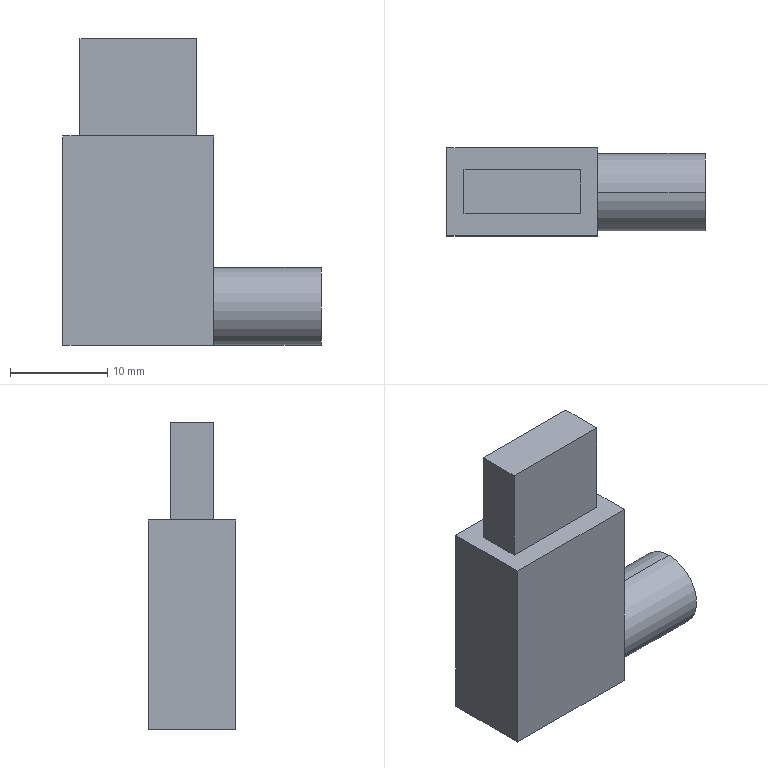Part | SolidWorks | features ICE 2, Extrusion 1 | 1 solid | 14 faces | box 26.5 x 9 x 31.5 mm | volume 4092 mm3 | plane 12 | cylinder 2 | commonest cylinder face diameters 8 x2
STEP:
#1=CARTESIAN_POINT('',(18.75,0.,-21.5));
#2=VERTEX_POINT('',#1);
#3=CARTESIAN_POINT('',(18.75,0.,-13.5));
#4=VERTEX_POINT('',#3);
#5=CARTESIAN_POINT('',(18.75,0.,-17.5));
#6=DIRECTION('',(1.,0.,0.));
#7=DIRECTION('',(0.,0.,-1.));
#8=AXIS2_PLACEMENT_3D('',#5,#6,#7);
#9=CIRCLE('',#8,4.);
#10=EDGE_CURVE('',#2,#4,#9,.T.);
#11=ORIENTED_EDGE('',*,*,#10,.F.);
#12=CARTESIAN_POINT('',(7.75,0.,-21.5));
#13=VERTEX_POINT('',#12);
#14=CARTESIAN_POINT('',(18.75,0.,-21.5));
#15=DIRECTION('',(-1.,0.,0.));
#16=VECTOR('',#15,1000.);
#17=LINE('',#14,#16);
#18=EDGE_CURVE('',#2,#13,#17,.T.);
#19=ORIENTED_EDGE('',*,*,#18,.T.);
#20=CARTESIAN_POINT('',(7.75,0.,-13.5));
#21=VERTEX_POINT('',#20);
#22=CARTESIAN_POINT('',(7.75,0.,-17.5));
#23=DIRECTION('',(1.,0.,0.));
#24=DIRECTION('',(0.,0.,-1.));
#25=AXIS2_PLACEMENT_3D('',#22,#23,#24);
#26=CIRCLE('',#25,4.);
#27=EDGE_CURVE('',#13,#21,#26,.T.);
#28=ORIENTED_EDGE('',*,*,#27,.T.);
#29=CARTESIAN_POINT('',(18.75,0.,-13.5));
#30=DIRECTION('',(-1.,0.,0.));
#31=VECTOR('',#30,1000.);
#32=LINE('',#29,#31);
#33=EDGE_CURVE('',#4,#21,#32,.T.);
#34=ORIENTED_EDGE('',*,*,#33,.F.);
#35=EDGE_LOOP('',(#11,#19,#28,#34));
#36=FACE_OUTER_BOUND('',#35,.T.);
#37=CARTESIAN_POINT('',(18.75,0.,-17.5));
#38=DIRECTION('',(-1.,0.,0.));
#39=DIRECTION('',(0.,0.,1.));
#40=AXIS2_PLACEMENT_3D('',#37,#38,#39);
#41=CYLINDRICAL_SURFACE('',#40,4.);
#42=ADVANCED_FACE('',(#36),#41,.T.);
#43=CARTESIAN_POINT('',(7.75,-4.5,0.));
#44=VERTEX_POINT('',#43);
#45=CARTESIAN_POINT('',(7.75,4.5,0.));
#46=VERTEX_POINT('',#45);
#47=CARTESIAN_POINT('',(7.75,-4.5,0.));
#48=DIRECTION('',(0.,1.,0.));
#49=VECTOR('',#48,1000.);
#50=LINE('',#47,#49);
#51=EDGE_CURVE('',#44,#46,#50,.T.);
#52=ORIENTED_EDGE('',*,*,#51,.T.);
#53=CARTESIAN_POINT('',(-7.75,4.5,0.));
#54=VERTEX_POINT('',#53);
#55=CARTESIAN_POINT('',(-7.75,4.5,0.));
#56=DIRECTION('',(-1.,0.,0.));
#57=VECTOR('',#56,1000.);
#58=LINE('',#55,#57);
#59=EDGE_CURVE('',#46,#54,#58,.T.);
#60=ORIENTED_EDGE('',*,*,#59,.T.);
#61=CARTESIAN_POINT('',(-7.75,-4.5,0.));
#62=VERTEX_POINT('',#61);
#63=CARTESIAN_POINT('',(-7.75,-4.5,0.));
#64=DIRECTION('',(0.,-1.,0.));
#65=VECTOR('',#64,1000.);
#66=LINE('',#63,#65);
#67=EDGE_CURVE('',#54,#62,#66,.T.);
#68=ORIENTED_EDGE('',*,*,#67,.T.);
#69=CARTESIAN_POINT('',(-7.75,-4.5,0.));
#70=DIRECTION('',(1.,0.,0.));
#71=VECTOR('',#70,1000.);
#72=LINE('',#69,#71);
#73=EDGE_CURVE('',#62,#44,#72,.T.);
#74=ORIENTED_EDGE('',*,*,#73,.T.);
#75=EDGE_LOOP('',(#52,#60,#68,#74));
#76=FACE_OUTER_BOUND('',#75,.T.);
#77=CARTESIAN_POINT('',(6.,-2.25,0.));
#78=VERTEX_POINT('',#77);
#79=CARTESIAN_POINT('',(6.,2.25,0.));
#80=VERTEX_POINT('',#79);
#81=CARTESIAN_POINT('',(6.,-2.25,0.));
#82=DIRECTION('',(0.,1.,0.));
#83=VECTOR('',#82,1000.);
#84=LINE('',#81,#83);
#85=EDGE_CURVE('',#78,#80,#84,.T.);
#86=ORIENTED_EDGE('',*,*,#85,.F.);
#87=CARTESIAN_POINT('',(-6.,-2.25,0.));
#88=VERTEX_POINT('',#87);
#89=CARTESIAN_POINT('',(-6.,-2.25,0.));
#90=DIRECTION('',(1.,0.,0.));
#91=VECTOR('',#90,1000.);
#92=LINE('',#89,#91);
#93=EDGE_CURVE('',#88,#78,#92,.T.);
#94=ORIENTED_EDGE('',*,*,#93,.F.);
#95=CARTESIAN_POINT('',(-6.,2.25,0.));
#96=VERTEX_POINT('',#95);
#97=CARTESIAN_POINT('',(-6.,-2.25,0.));
#98=DIRECTION('',(0.,-1.,0.));
#99=VECTOR('',#98,1000.);
#100=LINE('',#97,#99);
#101=EDGE_CURVE('',#96,#88,#100,.T.);
#102=ORIENTED_EDGE('',*,*,#101,.F.);
#103=CARTESIAN_POINT('',(-6.,2.25,0.));
#104=DIRECTION('',(-1.,0.,0.));
#105=VECTOR('',#104,1000.);
#106=LINE('',#103,#105);
#107=EDGE_CURVE('',#80,#96,#106,.T.);
#108=ORIENTED_EDGE('',*,*,#107,.F.);
#109=EDGE_LOOP('',(#86,#94,#102,#108));
#110=FACE_BOUND('',#109,.T.);
#111=CARTESIAN_POINT('',(0.,0.,0.));
#112=DIRECTION('',(0.,0.,-1.));
#113=DIRECTION('',(-1.,0.,0.));
#114=AXIS2_PLACEMENT_3D('',#111,#112,#113);
#115=PLANE('',#114);
#116=ADVANCED_FACE('',(#76,#110),#115,.F.);
#117=CARTESIAN_POINT('',(7.75,-4.5,-21.5));
#118=VERTEX_POINT('',#117);
#119=CARTESIAN_POINT('',(7.75,-4.5,-21.5));
#120=DIRECTION('',(0.,1.,0.));
#121=VECTOR('',#120,1000.);
#122=LINE('',#119,#121);
#123=EDGE_CURVE('',#118,#13,#122,.T.);
#124=ORIENTED_EDGE('',*,*,#123,.T.);
#125=CARTESIAN_POINT('',(7.75,0.,-17.5));
#126=DIRECTION('',(1.,0.,0.));
#127=DIRECTION('',(0.,0.,-1.));
#128=AXIS2_PLACEMENT_3D('',#125,#126,#127);
#129=CIRCLE('',#128,4.);
#130=EDGE_CURVE('',#21,#13,#129,.T.);
#131=ORIENTED_EDGE('',*,*,#130,.F.);
#132=ORIENTED_EDGE('',*,*,#27,.F.);
#133=CARTESIAN_POINT('',(7.75,4.5,-21.5));
#134=VERTEX_POINT('',#133);
#135=CARTESIAN_POINT('',(7.75,-4.5,-21.5));
#136=DIRECTION('',(0.,1.,0.));
#137=VECTOR('',#136,1000.);
#138=LINE('',#135,#137);
#139=EDGE_CURVE('',#13,#134,#138,.T.);
#140=ORIENTED_EDGE('',*,*,#139,.T.);
#141=CARTESIAN_POINT('',(7.75,4.5,-21.5));
#142=DIRECTION('',(0.,0.,1.));
#143=VECTOR('',#142,1000.);
#144=LINE('',#141,#143);
#145=EDGE_CURVE('',#134,#46,#144,.T.);
#146=ORIENTED_EDGE('',*,*,#145,.T.);
#147=ORIENTED_EDGE('',*,*,#51,.F.);
#148=CARTESIAN_POINT('',(7.75,-4.5,-21.5));
#149=DIRECTION('',(0.,0.,1.));
#150=VECTOR('',#149,1000.);
#151=LINE('',#148,#150);
#152=EDGE_CURVE('',#118,#44,#151,.T.);
#153=ORIENTED_EDGE('',*,*,#152,.F.);
#154=EDGE_LOOP('',(#124,#131,#132,#140,#146,#147,#153));
#155=FACE_OUTER_BOUND('',#154,.T.);
#156=CARTESIAN_POINT('',(7.75,-4.5,-21.5));
#157=DIRECTION('',(1.,0.,0.));
#158=DIRECTION('',(0.,0.,-1.));
#159=AXIS2_PLACEMENT_3D('',#156,#157,#158);
#160=PLANE('',#159);
#161=ADVANCED_FACE('',(#155),#160,.T.);
#162=ORIENTED_EDGE('',*,*,#73,.F.);
#163=CARTESIAN_POINT('',(-7.75,-4.5,-21.5));
#164=VERTEX_POINT('',#163);
#165=CARTESIAN_POINT('',(-7.75,-4.5,-21.5));
#166=DIRECTION('',(0.,0.,1.));
#167=VECTOR('',#166,1000.);
#168=LINE('',#165,#167);
#169=EDGE_CURVE('',#164,#62,#168,.T.);
#170=ORIENTED_EDGE('',*,*,#169,.F.);
#171=CARTESIAN_POINT('',(-7.75,-4.5,-21.5));
#172=DIRECTION('',(1.,0.,0.));
#173=VECTOR('',#172,1000.);
#174=LINE('',#171,#173);
#175=EDGE_CURVE('',#164,#118,#174,.T.);
#176=ORIENTED_EDGE('',*,*,#175,.T.);
#177=ORIENTED_EDGE('',*,*,#152,.T.);
#178=EDGE_LOOP('',(#162,#170,#176,#177));
#179=FACE_OUTER_BOUND('',#178,.T.);
#180=CARTESIAN_POINT('',(-7.75,-4.5,-21.5));
#181=DIRECTION('',(0.,-1.,0.));
#182=DIRECTION('',(0.,0.,-1.));
#183=AXIS2_PLACEMENT_3D('',#180,#181,#182);
#184=PLANE('',#183);
#185=ADVANCED_FACE('',(#179),#184,.T.);
#186=ORIENTED_EDGE('',*,*,#67,.F.);
#187=CARTESIAN_POINT('',(-7.75,4.5,-21.5));
#188=VERTEX_POINT('',#187);
#189=CARTESIAN_POINT('',(-7.75,4.5,-21.5));
#190=DIRECTION('',(0.,0.,1.));
#191=VECTOR('',#190,1000.);
#192=LINE('',#189,#191);
#193=EDGE_CURVE('',#188,#54,#192,.T.);
#194=ORIENTED_EDGE('',*,*,#193,.F.);
#195=CARTESIAN_POINT('',(-7.75,-4.5,-21.5));
#196=DIRECTION('',(0.,-1.,0.));
#197=VECTOR('',#196,1000.);
#198=LINE('',#195,#197);
#199=EDGE_CURVE('',#188,#164,#198,.T.);
#200=ORIENTED_EDGE('',*,*,#199,.T.);
#201=ORIENTED_EDGE('',*,*,#169,.T.);
#202=EDGE_LOOP('',(#186,#194,#200,#201));
#203=FACE_OUTER_BOUND('',#202,.T.);
#204=CARTESIAN_POINT('',(-7.75,-4.5,-21.5));
#205=DIRECTION('',(-1.,0.,0.));
#206=DIRECTION('',(0.,0.,1.));
#207=AXIS2_PLACEMENT_3D('',#204,#205,#206);
#208=PLANE('',#207);
#209=ADVANCED_FACE('',(#203),#208,.T.);
#210=ORIENTED_EDGE('',*,*,#59,.F.);
#211=ORIENTED_EDGE('',*,*,#145,.F.);
#212=CARTESIAN_POINT('',(-7.75,4.5,-21.5));
#213=DIRECTION('',(-1.,0.,0.));
#214=VECTOR('',#213,1000.);
#215=LINE('',#212,#214);
#216=EDGE_CURVE('',#134,#188,#215,.T.);
#217=ORIENTED_EDGE('',*,*,#216,.T.);
#218=ORIENTED_EDGE('',*,*,#193,.T.);
#219=EDGE_LOOP('',(#210,#211,#217,#218));
#220=FACE_OUTER_BOUND('',#219,.T.);
#221=CARTESIAN_POINT('',(-7.75,4.5,-21.5));
#222=DIRECTION('',(0.,1.,0.));
#223=DIRECTION('',(0.,0.,1.));
#224=AXIS2_PLACEMENT_3D('',#221,#222,#223);
#225=PLANE('',#224);
#226=ADVANCED_FACE('',(#220),#225,.T.);
#227=ORIENTED_EDGE('',*,*,#123,.F.);
#228=ORIENTED_EDGE('',*,*,#175,.F.);
#229=ORIENTED_EDGE('',*,*,#199,.F.);
#230=ORIENTED_EDGE('',*,*,#216,.F.);
#231=ORIENTED_EDGE('',*,*,#139,.F.);
#232=EDGE_LOOP('',(#227,#228,#229,#230,#231));
#233=FACE_OUTER_BOUND('',#232,.T.);
#234=CARTESIAN_POINT('',(0.,0.,-21.5));
#235=DIRECTION('',(0.,0.,-1.));
#236=DIRECTION('',(-1.,0.,0.));
#237=AXIS2_PLACEMENT_3D('',#234,#235,#236);
#238=PLANE('',#237);
#239=ADVANCED_FACE('',(#233),#238,.T.);
#240=ORIENTED_EDGE('',*,*,#18,.F.);
#241=CARTESIAN_POINT('',(18.75,0.,-17.5));
#242=DIRECTION('',(1.,0.,0.));
#243=DIRECTION('',(0.,0.,-1.));
#244=AXIS2_PLACEMENT_3D('',#241,#242,#243);
#245=CIRCLE('',#244,4.);
#246=EDGE_CURVE('',#4,#2,#245,.T.);
#247=ORIENTED_EDGE('',*,*,#246,.F.);
#248=ORIENTED_EDGE('',*,*,#33,.T.);
#249=ORIENTED_EDGE('',*,*,#130,.T.);
#250=EDGE_LOOP('',(#240,#247,#248,#249));
#251=FACE_OUTER_BOUND('',#250,.T.);
#252=CARTESIAN_POINT('',(18.75,0.,-17.5));
#253=DIRECTION('',(-1.,0.,0.));
#254=DIRECTION('',(0.,0.,1.));
#255=AXIS2_PLACEMENT_3D('',#252,#253,#254);
#256=CYLINDRICAL_SURFACE('',#255,4.);
#257=ADVANCED_FACE('',(#251),#256,.T.);
#258=ORIENTED_EDGE('',*,*,#246,.T.);
#259=ORIENTED_EDGE('',*,*,#10,.T.);
#260=EDGE_LOOP('',(#258,#259));
#261=FACE_OUTER_BOUND('',#260,.T.);
#262=CARTESIAN_POINT('',(18.75,0.,-17.5));
#263=DIRECTION('',(1.,0.,0.));
#264=DIRECTION('',(0.,0.,-1.));
#265=AXIS2_PLACEMENT_3D('',#262,#263,#264);
#266=PLANE('',#265);
#267=ADVANCED_FACE('',(#261),#266,.T.);
#268=ORIENTED_EDGE('',*,*,#85,.T.);
#269=CARTESIAN_POINT('',(6.,2.25,10.));
#270=VERTEX_POINT('',#269);
#271=CARTESIAN_POINT('',(6.,2.25,10.));
#272=DIRECTION('',(0.,0.,-1.));
#273=VECTOR('',#272,1000.);
#274=LINE('',#271,#273);
#275=EDGE_CURVE('',#270,#80,#274,.T.);
#276=ORIENTED_EDGE('',*,*,#275,.F.);
#277=CARTESIAN_POINT('',(6.,-2.25,10.));
#278=VERTEX_POINT('',#277);
#279=CARTESIAN_POINT('',(6.,-2.25,10.));
#280=DIRECTION('',(0.,1.,0.));
#281=VECTOR('',#280,1000.);
#282=LINE('',#279,#281);
#283=EDGE_CURVE('',#278,#270,#282,.T.);
#284=ORIENTED_EDGE('',*,*,#283,.F.);
#285=CARTESIAN_POINT('',(6.,-2.25,10.));
#286=DIRECTION('',(0.,0.,-1.));
#287=VECTOR('',#286,1000.);
#288=LINE('',#285,#287);
#289=EDGE_CURVE('',#278,#78,#288,.T.);
#290=ORIENTED_EDGE('',*,*,#289,.T.);
#291=EDGE_LOOP('',(#268,#276,#284,#290));
#292=FACE_OUTER_BOUND('',#291,.T.);
#293=CARTESIAN_POINT('',(6.,-2.25,10.));
#294=DIRECTION('',(-1.,0.,0.));
#295=DIRECTION('',(0.,0.,1.));
#296=AXIS2_PLACEMENT_3D('',#293,#294,#295);
#297=PLANE('',#296);
#298=ADVANCED_FACE('',(#292),#297,.F.);
#299=ORIENTED_EDGE('',*,*,#107,.T.);
#300=CARTESIAN_POINT('',(-6.,2.25,10.));
#301=VERTEX_POINT('',#300);
#302=CARTESIAN_POINT('',(-6.,2.25,10.));
#303=DIRECTION('',(0.,0.,-1.));
#304=VECTOR('',#303,1000.);
#305=LINE('',#302,#304);
#306=EDGE_CURVE('',#301,#96,#305,.T.);
#307=ORIENTED_EDGE('',*,*,#306,.F.);
#308=CARTESIAN_POINT('',(-6.,2.25,10.));
#309=DIRECTION('',(-1.,0.,0.));
#310=VECTOR('',#309,1000.);
#311=LINE('',#308,#310);
#312=EDGE_CURVE('',#270,#301,#311,.T.);
#313=ORIENTED_EDGE('',*,*,#312,.F.);
#314=ORIENTED_EDGE('',*,*,#275,.T.);
#315=EDGE_LOOP('',(#299,#307,#313,#314));
#316=FACE_OUTER_BOUND('',#315,.T.);
#317=CARTESIAN_POINT('',(-6.,2.25,10.));
#318=DIRECTION('',(0.,-1.,0.));
#319=DIRECTION('',(0.,0.,-1.));
#320=AXIS2_PLACEMENT_3D('',#317,#318,#319);
#321=PLANE('',#320);
#322=ADVANCED_FACE('',(#316),#321,.F.);
#323=ORIENTED_EDGE('',*,*,#101,.T.);
#324=CARTESIAN_POINT('',(-6.,-2.25,10.));
#325=VERTEX_POINT('',#324);
#326=CARTESIAN_POINT('',(-6.,-2.25,10.));
#327=DIRECTION('',(0.,0.,-1.));
#328=VECTOR('',#327,1000.);
#329=LINE('',#326,#328);
#330=EDGE_CURVE('',#325,#88,#329,.T.);
#331=ORIENTED_EDGE('',*,*,#330,.F.);
#332=CARTESIAN_POINT('',(-6.,-2.25,10.));
#333=DIRECTION('',(0.,-1.,0.));
#334=VECTOR('',#333,1000.);
#335=LINE('',#332,#334);
#336=EDGE_CURVE('',#301,#325,#335,.T.);
#337=ORIENTED_EDGE('',*,*,#336,.F.);
#338=ORIENTED_EDGE('',*,*,#306,.T.);
#339=EDGE_LOOP('',(#323,#331,#337,#338));
#340=FACE_OUTER_BOUND('',#339,.T.);
#341=CARTESIAN_POINT('',(-6.,-2.25,10.));
#342=DIRECTION('',(1.,0.,0.));
#343=DIRECTION('',(0.,0.,-1.));
#344=AXIS2_PLACEMENT_3D('',#341,#342,#343);
#345=PLANE('',#344);
#346=ADVANCED_FACE('',(#340),#345,.F.);
#347=ORIENTED_EDGE('',*,*,#93,.T.);
#348=ORIENTED_EDGE('',*,*,#289,.F.);
#349=CARTESIAN_POINT('',(-6.,-2.25,10.));
#350=DIRECTION('',(1.,0.,0.));
#351=VECTOR('',#350,1000.);
#352=LINE('',#349,#351);
#353=EDGE_CURVE('',#325,#278,#352,.T.);
#354=ORIENTED_EDGE('',*,*,#353,.F.);
#355=ORIENTED_EDGE('',*,*,#330,.T.);
#356=EDGE_LOOP('',(#347,#348,#354,#355));
#357=FACE_OUTER_BOUND('',#356,.T.);
#358=CARTESIAN_POINT('',(-6.,-2.25,10.));
#359=DIRECTION('',(0.,1.,0.));
#360=DIRECTION('',(0.,0.,1.));
#361=AXIS2_PLACEMENT_3D('',#358,#359,#360);
#362=PLANE('',#361);
#363=ADVANCED_FACE('',(#357),#362,.F.);
#364=ORIENTED_EDGE('',*,*,#283,.T.);
#365=ORIENTED_EDGE('',*,*,#312,.T.);
#366=ORIENTED_EDGE('',*,*,#336,.T.);
#367=ORIENTED_EDGE('',*,*,#353,.T.);
#368=EDGE_LOOP('',(#364,#365,#366,#367));
#369=FACE_OUTER_BOUND('',#368,.T.);
#370=CARTESIAN_POINT('',(0.,0.,10.));
#371=DIRECTION('',(0.,0.,-1.));
#372=DIRECTION('',(-1.,0.,0.));
#373=AXIS2_PLACEMENT_3D('',#370,#371,#372);
#374=PLANE('',#373);
#375=ADVANCED_FACE('',(#369),#374,.F.);
#376=CLOSED_SHELL('',(#42,#116,#161,#185,#209,#226,#239,#257,#267,#298,#322,#346,#363,#375));
#377=MANIFOLD_SOLID_BREP('',#376);
#378=CARTESIAN_POINT('',(0.,0.,0.));
#379=DIRECTION('',(0.,0.,1.));
#380=DIRECTION('',(1.,0.,0.));
#381=AXIS2_PLACEMENT_3D('',#378,#379,#380);
#382=(LENGTH_UNIT()NAMED_UNIT(*)SI_UNIT(.MILLI.,.METRE.));
#383=UNCERTAINTY_MEASURE_WITH_UNIT(LENGTH_MEASURE(0.00001),#382,'','');
#384=(NAMED_UNIT(*)PLANE_ANGLE_UNIT()SI_UNIT($,.RADIAN.));
#385=(NAMED_UNIT(*)SI_UNIT($,.STERADIAN.)SOLID_ANGLE_UNIT());
#386=(GEOMETRIC_REPRESENTATION_CONTEXT(3)GLOBAL_UNCERTAINTY_ASSIGNED_CONTEXT((#383))GLOBAL_UNIT_ASSIGNED_CONTEXT((#382,#384,#385))REPRESENTATION_CONTEXT('',''));
#387=ADVANCED_BREP_SHAPE_REPRESENTATION('',(#377,#381),#386);